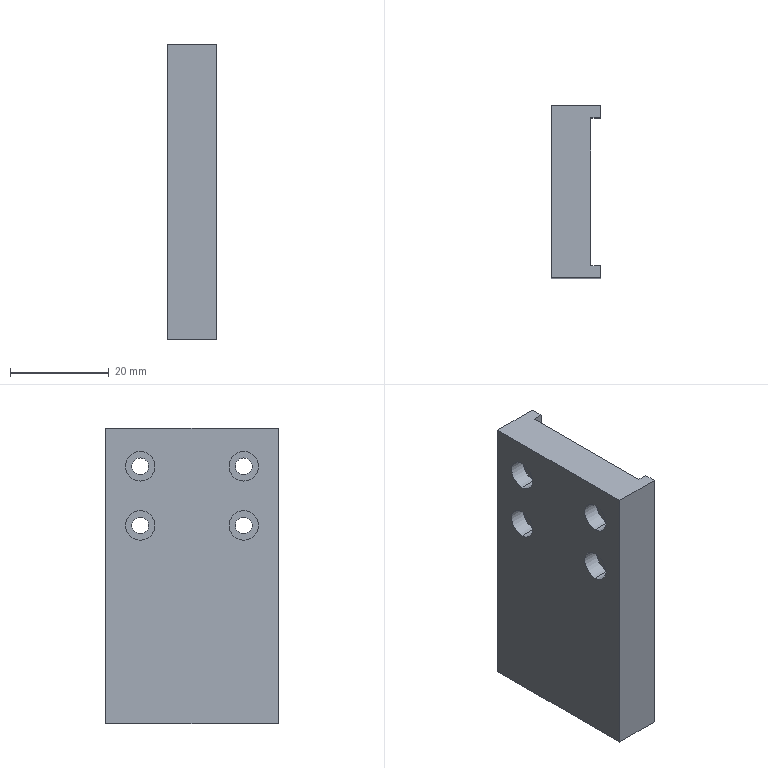Part | SolidWorks | features HoleWzd 2, Cut 1, Extrusion 1 | 1 solid | 38 faces | box 10 x 35 x 60 mm | volume 16670 mm3 | cylinder 20 | plane 14 | cone 4 | commonest cylinder face diameters 3.4 x8 6 x8 3.3 x4
STEP:
#1=CARTESIAN_POINT('',(5.65,10.,-19.9));
#2=VERTEX_POINT('',#1);
#3=CARTESIAN_POINT('',(2.35,10.,-19.9));
#4=VERTEX_POINT('',#3);
#5=CARTESIAN_POINT('',(4.,10.,-19.9));
#6=DIRECTION('',(0.,0.,-1.));
#7=DIRECTION('',(-1.,0.,0.));
#8=AXIS2_PLACEMENT_3D('',#5,#6,#7);
#9=CIRCLE('',#8,1.65);
#10=EDGE_CURVE('',#2,#4,#9,.T.);
#11=ORIENTED_EDGE('',*,*,#10,.F.);
#12=CARTESIAN_POINT('',(5.65,10.,-30.));
#13=VERTEX_POINT('',#12);
#14=CARTESIAN_POINT('',(5.65,10.,-30.));
#15=DIRECTION('',(0.,0.,-1.));
#16=VECTOR('',#15,1000.);
#17=LINE('',#14,#16);
#18=EDGE_CURVE('',#2,#13,#17,.T.);
#19=ORIENTED_EDGE('',*,*,#18,.T.);
#20=CARTESIAN_POINT('',(2.35,10.,-30.));
#21=VERTEX_POINT('',#20);
#22=CARTESIAN_POINT('',(4.,10.,-30.));
#23=DIRECTION('',(0.,0.,-1.));
#24=DIRECTION('',(-1.,0.,0.));
#25=AXIS2_PLACEMENT_3D('',#22,#23,#24);
#26=CIRCLE('',#25,1.65);
#27=EDGE_CURVE('',#13,#21,#26,.T.);
#28=ORIENTED_EDGE('',*,*,#27,.T.);
#29=CARTESIAN_POINT('',(2.35,10.,-30.));
#30=DIRECTION('',(0.,0.,-1.));
#31=VECTOR('',#30,1000.);
#32=LINE('',#29,#31);
#33=EDGE_CURVE('',#4,#21,#32,.T.);
#34=ORIENTED_EDGE('',*,*,#33,.F.);
#35=EDGE_LOOP('',(#11,#19,#28,#34));
#36=FACE_OUTER_BOUND('',#35,.T.);
#37=CARTESIAN_POINT('',(4.,10.,-30.));
#38=DIRECTION('',(0.,0.,-1.));
#39=DIRECTION('',(-1.,0.,0.));
#40=AXIS2_PLACEMENT_3D('',#37,#38,#39);
#41=CYLINDRICAL_SURFACE('',#40,1.65);
#42=ADVANCED_FACE('',(#36),#41,.F.);
#43=CARTESIAN_POINT('',(4.,10.,-18.909));
#44=VERTEX_POINT('',#43);
#45=CARTESIAN_POINT('',(2.35,10.,-19.9));
#46=DIRECTION('',(-0.8572,0.,-0.515));
#47=VECTOR('',#46,1000.);
#48=LINE('',#45,#47);
#49=EDGE_CURVE('',#44,#4,#48,.T.);
#50=ORIENTED_EDGE('',*,*,#49,.F.);
#51=CARTESIAN_POINT('',(5.65,10.,-19.9));
#52=DIRECTION('',(0.8572,0.,-0.515));
#53=VECTOR('',#52,1000.);
#54=LINE('',#51,#53);
#55=EDGE_CURVE('',#44,#2,#54,.T.);
#56=ORIENTED_EDGE('',*,*,#55,.T.);
#57=ORIENTED_EDGE('',*,*,#10,.T.);
#58=EDGE_LOOP('',(#50,#56,#57));
#59=FACE_OUTER_BOUND('',#58,.T.);
#60=CARTESIAN_POINT('',(4.,10.,-19.9));
#61=DIRECTION('',(0.,0.,-1.));
#62=DIRECTION('',(-1.,0.,0.));
#63=AXIS2_PLACEMENT_3D('',#60,#61,#62);
#64=CONICAL_SURFACE('',#63,1.65,1.03);
#65=ADVANCED_FACE('',(#59),#64,.F.);
#66=CARTESIAN_POINT('',(5.65,-10.,-19.9));
#67=VERTEX_POINT('',#66);
#68=CARTESIAN_POINT('',(2.35,-10.,-19.9));
#69=VERTEX_POINT('',#68);
#70=CARTESIAN_POINT('',(4.,-10.,-19.9));
#71=DIRECTION('',(0.,0.,-1.));
#72=DIRECTION('',(-1.,0.,0.));
#73=AXIS2_PLACEMENT_3D('',#70,#71,#72);
#74=CIRCLE('',#73,1.65);
#75=EDGE_CURVE('',#67,#69,#74,.T.);
#76=ORIENTED_EDGE('',*,*,#75,.F.);
#77=CARTESIAN_POINT('',(5.65,-10.,-30.));
#78=VERTEX_POINT('',#77);
#79=CARTESIAN_POINT('',(5.65,-10.,-30.));
#80=DIRECTION('',(0.,0.,-1.));
#81=VECTOR('',#80,1000.);
#82=LINE('',#79,#81);
#83=EDGE_CURVE('',#67,#78,#82,.T.);
#84=ORIENTED_EDGE('',*,*,#83,.T.);
#85=CARTESIAN_POINT('',(2.35,-10.,-30.));
#86=VERTEX_POINT('',#85);
#87=CARTESIAN_POINT('',(4.,-10.,-30.));
#88=DIRECTION('',(0.,0.,-1.));
#89=DIRECTION('',(-1.,0.,0.));
#90=AXIS2_PLACEMENT_3D('',#87,#88,#89);
#91=CIRCLE('',#90,1.65);
#92=EDGE_CURVE('',#78,#86,#91,.T.);
#93=ORIENTED_EDGE('',*,*,#92,.T.);
#94=CARTESIAN_POINT('',(2.35,-10.,-30.));
#95=DIRECTION('',(0.,0.,-1.));
#96=VECTOR('',#95,1000.);
#97=LINE('',#94,#96);
#98=EDGE_CURVE('',#69,#86,#97,.T.);
#99=ORIENTED_EDGE('',*,*,#98,.F.);
#100=EDGE_LOOP('',(#76,#84,#93,#99));
#101=FACE_OUTER_BOUND('',#100,.T.);
#102=CARTESIAN_POINT('',(4.,-10.,-30.));
#103=DIRECTION('',(0.,0.,-1.));
#104=DIRECTION('',(-1.,0.,0.));
#105=AXIS2_PLACEMENT_3D('',#102,#103,#104);
#106=CYLINDRICAL_SURFACE('',#105,1.65);
#107=ADVANCED_FACE('',(#101),#106,.F.);
#108=CARTESIAN_POINT('',(4.,-10.,-18.909));
#109=VERTEX_POINT('',#108);
#110=CARTESIAN_POINT('',(2.35,-10.,-19.9));
#111=DIRECTION('',(-0.8572,0.,-0.515));
#112=VECTOR('',#111,1000.);
#113=LINE('',#110,#112);
#114=EDGE_CURVE('',#109,#69,#113,.T.);
#115=ORIENTED_EDGE('',*,*,#114,.F.);
#116=CARTESIAN_POINT('',(5.65,-10.,-19.9));
#117=DIRECTION('',(0.8572,0.,-0.515));
#118=VECTOR('',#117,1000.);
#119=LINE('',#116,#118);
#120=EDGE_CURVE('',#109,#67,#119,.T.);
#121=ORIENTED_EDGE('',*,*,#120,.T.);
#122=ORIENTED_EDGE('',*,*,#75,.T.);
#123=EDGE_LOOP('',(#115,#121,#122));
#124=FACE_OUTER_BOUND('',#123,.T.);
#125=CARTESIAN_POINT('',(4.,-10.,-19.9));
#126=DIRECTION('',(0.,0.,-1.));
#127=DIRECTION('',(-1.,0.,0.));
#128=AXIS2_PLACEMENT_3D('',#125,#126,#127);
#129=CONICAL_SURFACE('',#128,1.65,1.03);
#130=ADVANCED_FACE('',(#124),#129,.F.);
#131=CARTESIAN_POINT('',(3.4,10.5,19.25));
#132=VERTEX_POINT('',#131);
#133=CARTESIAN_POINT('',(3.4,10.5,25.25));
#134=VERTEX_POINT('',#133);
#135=CARTESIAN_POINT('',(3.4,10.5,22.25));
#136=DIRECTION('',(-1.,0.,0.));
#137=DIRECTION('',(0.,0.,1.));
#138=AXIS2_PLACEMENT_3D('',#135,#136,#137);
#139=CIRCLE('',#138,3.);
#140=EDGE_CURVE('',#132,#134,#139,.T.);
#141=ORIENTED_EDGE('',*,*,#140,.F.);
#142=CARTESIAN_POINT('',(0.,10.5,19.25));
#143=VERTEX_POINT('',#142);
#144=CARTESIAN_POINT('',(0.,10.5,19.25));
#145=DIRECTION('',(-1.,0.,0.));
#146=VECTOR('',#145,1000.);
#147=LINE('',#144,#146);
#148=EDGE_CURVE('',#132,#143,#147,.T.);
#149=ORIENTED_EDGE('',*,*,#148,.T.);
#150=CARTESIAN_POINT('',(0.,10.5,25.25));
#151=VERTEX_POINT('',#150);
#152=CARTESIAN_POINT('',(0.,10.5,22.25));
#153=DIRECTION('',(-1.,0.,0.));
#154=DIRECTION('',(0.,0.,1.));
#155=AXIS2_PLACEMENT_3D('',#152,#153,#154);
#156=CIRCLE('',#155,3.);
#157=EDGE_CURVE('',#143,#151,#156,.T.);
#158=ORIENTED_EDGE('',*,*,#157,.T.);
#159=CARTESIAN_POINT('',(0.,10.5,25.25));
#160=DIRECTION('',(-1.,0.,0.));
#161=VECTOR('',#160,1000.);
#162=LINE('',#159,#161);
#163=EDGE_CURVE('',#134,#151,#162,.T.);
#164=ORIENTED_EDGE('',*,*,#163,.F.);
#165=EDGE_LOOP('',(#141,#149,#158,#164));
#166=FACE_OUTER_BOUND('',#165,.T.);
#167=CARTESIAN_POINT('',(0.,10.5,22.25));
#168=DIRECTION('',(-1.,0.,0.));
#169=DIRECTION('',(0.,0.,1.));
#170=AXIS2_PLACEMENT_3D('',#167,#168,#169);
#171=CYLINDRICAL_SURFACE('',#170,3.);
#172=ADVANCED_FACE('',(#166),#171,.F.);
#173=CARTESIAN_POINT('',(8.,10.5,23.95));
#174=VERTEX_POINT('',#173);
#175=CARTESIAN_POINT('',(8.,10.5,20.55));
#176=VERTEX_POINT('',#175);
#177=CARTESIAN_POINT('',(8.,10.5,22.25));
#178=DIRECTION('',(1.,0.,0.));
#179=DIRECTION('',(0.,0.,-1.));
#180=AXIS2_PLACEMENT_3D('',#177,#178,#179);
#181=CIRCLE('',#180,1.7);
#182=EDGE_CURVE('',#174,#176,#181,.T.);
#183=ORIENTED_EDGE('',*,*,#182,.T.);
#184=CARTESIAN_POINT('',(3.4,10.5,20.55));
#185=VERTEX_POINT('',#184);
#186=CARTESIAN_POINT('',(0.,10.5,20.55));
#187=DIRECTION('',(-1.,0.,0.));
#188=VECTOR('',#187,1000.);
#189=LINE('',#186,#188);
#190=EDGE_CURVE('',#176,#185,#189,.T.);
#191=ORIENTED_EDGE('',*,*,#190,.T.);
#192=CARTESIAN_POINT('',(3.4,10.5,23.95));
#193=VERTEX_POINT('',#192);
#194=CARTESIAN_POINT('',(3.4,10.5,22.25));
#195=DIRECTION('',(-1.,0.,0.));
#196=DIRECTION('',(0.,0.,1.));
#197=AXIS2_PLACEMENT_3D('',#194,#195,#196);
#198=CIRCLE('',#197,1.7);
#199=EDGE_CURVE('',#185,#193,#198,.T.);
#200=ORIENTED_EDGE('',*,*,#199,.T.);
#201=CARTESIAN_POINT('',(0.,10.5,23.95));
#202=DIRECTION('',(-1.,0.,0.));
#203=VECTOR('',#202,1000.);
#204=LINE('',#201,#203);
#205=EDGE_CURVE('',#174,#193,#204,.T.);
#206=ORIENTED_EDGE('',*,*,#205,.F.);
#207=EDGE_LOOP('',(#183,#191,#200,#206));
#208=FACE_OUTER_BOUND('',#207,.T.);
#209=CARTESIAN_POINT('',(0.,10.5,22.25));
#210=DIRECTION('',(-1.,0.,0.));
#211=DIRECTION('',(0.,0.,1.));
#212=AXIS2_PLACEMENT_3D('',#209,#210,#211);
#213=CYLINDRICAL_SURFACE('',#212,1.7);
#214=ADVANCED_FACE('',(#208),#213,.F.);
#215=CARTESIAN_POINT('',(3.4,10.5,7.25));
#216=VERTEX_POINT('',#215);
#217=CARTESIAN_POINT('',(3.4,10.5,13.25));
#218=VERTEX_POINT('',#217);
#219=CARTESIAN_POINT('',(3.4,10.5,10.25));
#220=DIRECTION('',(-1.,0.,0.));
#221=DIRECTION('',(0.,0.,1.));
#222=AXIS2_PLACEMENT_3D('',#219,#220,#221);
#223=CIRCLE('',#222,3.);
#224=EDGE_CURVE('',#216,#218,#223,.T.);
#225=ORIENTED_EDGE('',*,*,#224,.F.);
#226=CARTESIAN_POINT('',(0.,10.5,7.25));
#227=VERTEX_POINT('',#226);
#228=CARTESIAN_POINT('',(0.,10.5,7.25));
#229=DIRECTION('',(-1.,0.,0.));
#230=VECTOR('',#229,1000.);
#231=LINE('',#228,#230);
#232=EDGE_CURVE('',#216,#227,#231,.T.);
#233=ORIENTED_EDGE('',*,*,#232,.T.);
#234=CARTESIAN_POINT('',(0.,10.5,13.25));
#235=VERTEX_POINT('',#234);
#236=CARTESIAN_POINT('',(0.,10.5,10.25));
#237=DIRECTION('',(-1.,0.,0.));
#238=DIRECTION('',(0.,0.,1.));
#239=AXIS2_PLACEMENT_3D('',#236,#237,#238);
#240=CIRCLE('',#239,3.);
#241=EDGE_CURVE('',#227,#235,#240,.T.);
#242=ORIENTED_EDGE('',*,*,#241,.T.);
#243=CARTESIAN_POINT('',(0.,10.5,13.25));
#244=DIRECTION('',(-1.,0.,0.));
#245=VECTOR('',#244,1000.);
#246=LINE('',#243,#245);
#247=EDGE_CURVE('',#218,#235,#246,.T.);
#248=ORIENTED_EDGE('',*,*,#247,.F.);
#249=EDGE_LOOP('',(#225,#233,#242,#248));
#250=FACE_OUTER_BOUND('',#249,.T.);
#251=CARTESIAN_POINT('',(0.,10.5,10.25));
#252=DIRECTION('',(-1.,0.,0.));
#253=DIRECTION('',(0.,0.,1.));
#254=AXIS2_PLACEMENT_3D('',#251,#252,#253);
#255=CYLINDRICAL_SURFACE('',#254,3.);
#256=ADVANCED_FACE('',(#250),#255,.F.);
#257=CARTESIAN_POINT('',(8.,10.5,11.95));
#258=VERTEX_POINT('',#257);
#259=CARTESIAN_POINT('',(8.,10.5,8.55));
#260=VERTEX_POINT('',#259);
#261=CARTESIAN_POINT('',(8.,10.5,10.25));
#262=DIRECTION('',(1.,0.,0.));
#263=DIRECTION('',(0.,0.,-1.));
#264=AXIS2_PLACEMENT_3D('',#261,#262,#263);
#265=CIRCLE('',#264,1.7);
#266=EDGE_CURVE('',#258,#260,#265,.T.);
#267=ORIENTED_EDGE('',*,*,#266,.T.);
#268=CARTESIAN_POINT('',(3.4,10.5,8.55));
#269=VERTEX_POINT('',#268);
#270=CARTESIAN_POINT('',(0.,10.5,8.55));
#271=DIRECTION('',(-1.,0.,0.));
#272=VECTOR('',#271,1000.);
#273=LINE('',#270,#272);
#274=EDGE_CURVE('',#260,#269,#273,.T.);
#275=ORIENTED_EDGE('',*,*,#274,.T.);
#276=CARTESIAN_POINT('',(3.4,10.5,11.95));
#277=VERTEX_POINT('',#276);
#278=CARTESIAN_POINT('',(3.4,10.5,10.25));
#279=DIRECTION('',(-1.,0.,0.));
#280=DIRECTION('',(0.,0.,1.));
#281=AXIS2_PLACEMENT_3D('',#278,#279,#280);
#282=CIRCLE('',#281,1.7);
#283=EDGE_CURVE('',#269,#277,#282,.T.);
#284=ORIENTED_EDGE('',*,*,#283,.T.);
#285=CARTESIAN_POINT('',(0.,10.5,11.95));
#286=DIRECTION('',(-1.,0.,0.));
#287=VECTOR('',#286,1000.);
#288=LINE('',#285,#287);
#289=EDGE_CURVE('',#258,#277,#288,.T.);
#290=ORIENTED_EDGE('',*,*,#289,.F.);
#291=EDGE_LOOP('',(#267,#275,#284,#290));
#292=FACE_OUTER_BOUND('',#291,.T.);
#293=CARTESIAN_POINT('',(0.,10.5,10.25));
#294=DIRECTION('',(-1.,0.,0.));
#295=DIRECTION('',(0.,0.,1.));
#296=AXIS2_PLACEMENT_3D('',#293,#294,#295);
#297=CYLINDRICAL_SURFACE('',#296,1.7);
#298=ADVANCED_FACE('',(#292),#297,.F.);
#299=CARTESIAN_POINT('',(3.4,-10.5,7.25));
#300=VERTEX_POINT('',#299);
#301=CARTESIAN_POINT('',(3.4,-10.5,13.25));
#302=VERTEX_POINT('',#301);
#303=CARTESIAN_POINT('',(3.4,-10.5,10.25));
#304=DIRECTION('',(-1.,0.,0.));
#305=DIRECTION('',(0.,0.,1.));
#306=AXIS2_PLACEMENT_3D('',#303,#304,#305);
#307=CIRCLE('',#306,3.);
#308=EDGE_CURVE('',#300,#302,#307,.T.);
#309=ORIENTED_EDGE('',*,*,#308,.F.);
#310=CARTESIAN_POINT('',(0.,-10.5,7.25));
#311=VERTEX_POINT('',#310);
#312=CARTESIAN_POINT('',(0.,-10.5,7.25));
#313=DIRECTION('',(-1.,0.,0.));
#314=VECTOR('',#313,1000.);
#315=LINE('',#312,#314);
#316=EDGE_CURVE('',#300,#311,#315,.T.);
#317=ORIENTED_EDGE('',*,*,#316,.T.);
#318=CARTESIAN_POINT('',(0.,-10.5,13.25));
#319=VERTEX_POINT('',#318);
#320=CARTESIAN_POINT('',(0.,-10.5,10.25));
#321=DIRECTION('',(-1.,0.,0.));
#322=DIRECTION('',(0.,0.,1.));
#323=AXIS2_PLACEMENT_3D('',#320,#321,#322);
#324=CIRCLE('',#323,3.);
#325=EDGE_CURVE('',#311,#319,#324,.T.);
#326=ORIENTED_EDGE('',*,*,#325,.T.);
#327=CARTESIAN_POINT('',(0.,-10.5,13.25));
#328=DIRECTION('',(-1.,0.,0.));
#329=VECTOR('',#328,1000.);
#330=LINE('',#327,#329);
#331=EDGE_CURVE('',#302,#319,#330,.T.);
#332=ORIENTED_EDGE('',*,*,#331,.F.);
#333=EDGE_LOOP('',(#309,#317,#326,#332));
#334=FACE_OUTER_BOUND('',#333,.T.);
#335=CARTESIAN_POINT('',(0.,-10.5,10.25));
#336=DIRECTION('',(-1.,0.,0.));
#337=DIRECTION('',(0.,0.,1.));
#338=AXIS2_PLACEMENT_3D('',#335,#336,#337);
#339=CYLINDRICAL_SURFACE('',#338,3.);
#340=ADVANCED_FACE('',(#334),#339,.F.);
#341=CARTESIAN_POINT('',(8.,-10.5,11.95));
#342=VERTEX_POINT('',#341);
#343=CARTESIAN_POINT('',(8.,-10.5,8.55));
#344=VERTEX_POINT('',#343);
#345=CARTESIAN_POINT('',(8.,-10.5,10.25));
#346=DIRECTION('',(1.,0.,0.));
#347=DIRECTION('',(0.,0.,-1.));
#348=AXIS2_PLACEMENT_3D('',#345,#346,#347);
#349=CIRCLE('',#348,1.7);
#350=EDGE_CURVE('',#342,#344,#349,.T.);
#351=ORIENTED_EDGE('',*,*,#350,.T.);
#352=CARTESIAN_POINT('',(3.4,-10.5,8.55));
#353=VERTEX_POINT('',#352);
#354=CARTESIAN_POINT('',(0.,-10.5,8.55));
#355=DIRECTION('',(-1.,0.,0.));
#356=VECTOR('',#355,1000.);
#357=LINE('',#354,#356);
#358=EDGE_CURVE('',#344,#353,#357,.T.);
#359=ORIENTED_EDGE('',*,*,#358,.T.);
#360=CARTESIAN_POINT('',(3.4,-10.5,11.95));
#361=VERTEX_POINT('',#360);
#362=CARTESIAN_POINT('',(3.4,-10.5,10.25));
#363=DIRECTION('',(-1.,0.,0.));
#364=DIRECTION('',(0.,0.,1.));
#365=AXIS2_PLACEMENT_3D('',#362,#363,#364);
#366=CIRCLE('',#365,1.7);
#367=EDGE_CURVE('',#353,#361,#366,.T.);
#368=ORIENTED_EDGE('',*,*,#367,.T.);
#369=CARTESIAN_POINT('',(0.,-10.5,11.95));
#370=DIRECTION('',(-1.,0.,0.));
#371=VECTOR('',#370,1000.);
#372=LINE('',#369,#371);
#373=EDGE_CURVE('',#342,#361,#372,.T.);
#374=ORIENTED_EDGE('',*,*,#373,.F.);
#375=EDGE_LOOP('',(#351,#359,#368,#374));
#376=FACE_OUTER_BOUND('',#375,.T.);
#377=CARTESIAN_POINT('',(0.,-10.5,10.25));
#378=DIRECTION('',(-1.,0.,0.));
#379=DIRECTION('',(0.,0.,1.));
#380=AXIS2_PLACEMENT_3D('',#377,#378,#379);
#381=CYLINDRICAL_SURFACE('',#380,1.7);
#382=ADVANCED_FACE('',(#376),#381,.F.);
#383=CARTESIAN_POINT('',(3.4,-10.5,19.25));
#384=VERTEX_POINT('',#383);
#385=CARTESIAN_POINT('',(3.4,-10.5,25.25));
#386=VERTEX_POINT('',#385);
#387=CARTESIAN_POINT('',(3.4,-10.5,22.25));
#388=DIRECTION('',(-1.,0.,0.));
#389=DIRECTION('',(0.,0.,1.));
#390=AXIS2_PLACEMENT_3D('',#387,#388,#389);
#391=CIRCLE('',#390,3.);
#392=EDGE_CURVE('',#384,#386,#391,.T.);
#393=ORIENTED_EDGE('',*,*,#392,.F.);
#394=CARTESIAN_POINT('',(0.,-10.5,19.25));
#395=VERTEX_POINT('',#394);
#396=CARTESIAN_POINT('',(0.,-10.5,19.25));
#397=DIRECTION('',(-1.,0.,0.));
#398=VECTOR('',#397,1000.);
#399=LINE('',#396,#398);
#400=EDGE_CURVE('',#384,#395,#399,.T.);
#401=ORIENTED_EDGE('',*,*,#400,.T.);
#402=CARTESIAN_POINT('',(0.,-10.5,25.25));
#403=VERTEX_POINT('',#402);
#404=CARTESIAN_POINT('',(0.,-10.5,22.25));
#405=DIRECTION('',(-1.,0.,0.));
#406=DIRECTION('',(0.,0.,1.));
#407=AXIS2_PLACEMENT_3D('',#404,#405,#406);
#408=CIRCLE('',#407,3.);
#409=EDGE_CURVE('',#395,#403,#408,.T.);
#410=ORIENTED_EDGE('',*,*,#409,.T.);
#411=CARTESIAN_POINT('',(0.,-10.5,25.25));
#412=DIRECTION('',(-1.,0.,0.));
#413=VECTOR('',#412,1000.);
#414=LINE('',#411,#413);
#415=EDGE_CURVE('',#386,#403,#414,.T.);
#416=ORIENTED_EDGE('',*,*,#415,.F.);
#417=EDGE_LOOP('',(#393,#401,#410,#416));
#418=FACE_OUTER_BOUND('',#417,.T.);
#419=CARTESIAN_POINT('',(0.,-10.5,22.25));
#420=DIRECTION('',(-1.,0.,0.));
#421=DIRECTION('',(0.,0.,1.));
#422=AXIS2_PLACEMENT_3D('',#419,#420,#421);
#423=CYLINDRICAL_SURFACE('',#422,3.);
#424=ADVANCED_FACE('',(#418),#423,.F.);
#425=CARTESIAN_POINT('',(8.,-10.5,23.95));
#426=VERTEX_POINT('',#425);
#427=CARTESIAN_POINT('',(8.,-10.5,20.55));
#428=VERTEX_POINT('',#427);
#429=CARTESIAN_POINT('',(8.,-10.5,22.25));
#430=DIRECTION('',(1.,0.,0.));
#431=DIRECTION('',(0.,0.,-1.));
#432=AXIS2_PLACEMENT_3D('',#429,#430,#431);
#433=CIRCLE('',#432,1.7);
#434=EDGE_CURVE('',#426,#428,#433,.T.);
#435=ORIENTED_EDGE('',*,*,#434,.T.);
#436=CARTESIAN_POINT('',(3.4,-10.5,20.55));
#437=VERTEX_POINT('',#436);
#438=CARTESIAN_POINT('',(0.,-10.5,20.55));
#439=DIRECTION('',(-1.,0.,0.));
#440=VECTOR('',#439,1000.);
#441=LINE('',#438,#440);
#442=EDGE_CURVE('',#428,#437,#441,.T.);
#443=ORIENTED_EDGE('',*,*,#442,.T.);
#444=CARTESIAN_POINT('',(3.4,-10.5,23.95));
#445=VERTEX_POINT('',#444);
#446=CARTESIAN_POINT('',(3.4,-10.5,22.25));
#447=DIRECTION('',(-1.,0.,0.));
#448=DIRECTION('',(0.,0.,1.));
#449=AXIS2_PLACEMENT_3D('',#446,#447,#448);
#450=CIRCLE('',#449,1.7);
#451=EDGE_CURVE('',#437,#445,#450,.T.);
#452=ORIENTED_EDGE('',*,*,#451,.T.);
#453=CARTESIAN_POINT('',(0.,-10.5,23.95));
#454=DIRECTION('',(-1.,0.,0.));
#455=VECTOR('',#454,1000.);
#456=LINE('',#453,#455);
#457=EDGE_CURVE('',#426,#445,#456,.T.);
#458=ORIENTED_EDGE('',*,*,#457,.F.);
#459=EDGE_LOOP('',(#435,#443,#452,#458));
#460=FACE_OUTER_BOUND('',#459,.T.);
#461=CARTESIAN_POINT('',(0.,-10.5,22.25));
#462=DIRECTION('',(-1.,0.,0.));
#463=DIRECTION('',(0.,0.,1.));
#464=AXIS2_PLACEMENT_3D('',#461,#462,#463);
#465=CYLINDRICAL_SURFACE('',#464,1.7);
#466=ADVANCED_FACE('',(#460),#465,.F.);
#467=CARTESIAN_POINT('',(10.,-17.5,-30.));
#468=VERTEX_POINT('',#467);
#469=CARTESIAN_POINT('',(10.,-15.,-30.));
#470=VERTEX_POINT('',#469);
#471=CARTESIAN_POINT('',(10.,-17.5,-30.));
#472=DIRECTION('',(0.,1.,0.));
#473=VECTOR('',#472,1000.);
#474=LINE('',#471,#473);
#475=EDGE_CURVE('',#468,#470,#474,.T.);
#476=ORIENTED_EDGE('',*,*,#475,.T.);
#477=CARTESIAN_POINT('',(10.,-15.,30.));
#478=VERTEX_POINT('',#477);
#479=CARTESIAN_POINT('',(10.,-15.,30.));
#480=DIRECTION('',(0.,0.,-1.));
#481=VECTOR('',#480,1000.);
#482=LINE('',#479,#481);
#483=EDGE_CURVE('',#478,#470,#482,.T.);
#484=ORIENTED_EDGE('',*,*,#483,.F.);
#485=CARTESIAN_POINT('',(10.,-17.5,30.));
#486=VERTEX_POINT('',#485);
#487=CARTESIAN_POINT('',(10.,-17.5,30.));
#488=DIRECTION('',(0.,-1.,0.));
#489=VECTOR('',#488,1000.);
#490=LINE('',#487,#489);
#491=EDGE_CURVE('',#478,#486,#490,.T.);
#492=ORIENTED_EDGE('',*,*,#491,.T.);
#493=CARTESIAN_POINT('',(10.,-17.5,30.));
#494=DIRECTION('',(0.,0.,-1.));
#495=VECTOR('',#494,1000.);
#496=LINE('',#493,#495);
#497=EDGE_CURVE('',#486,#468,#496,.T.);
#498=ORIENTED_EDGE('',*,*,#497,.T.);
#499=EDGE_LOOP('',(#476,#484,#492,#498));
#500=FACE_OUTER_BOUND('',#499,.T.);
#501=CARTESIAN_POINT('',(10.,0.,0.));
#502=DIRECTION('',(-1.,0.,0.));
#503=DIRECTION('',(0.,0.,1.));
#504=AXIS2_PLACEMENT_3D('',#501,#502,#503);
#505=PLANE('',#504);
#506=ADVANCED_FACE('',(#500),#505,.F.);
#507=CARTESIAN_POINT('',(4.,10.,-30.));
#508=DIRECTION('',(0.,0.,-1.));
#509=DIRECTION('',(-1.,0.,0.));
#510=AXIS2_PLACEMENT_3D('',#507,#508,#509);
#511=CIRCLE('',#510,1.65);
#512=EDGE_CURVE('',#21,#13,#511,.T.);
#513=ORIENTED_EDGE('',*,*,#512,.F.);
#514=ORIENTED_EDGE('',*,*,#27,.F.);
#515=EDGE_LOOP('',(#513,#514));
#516=FACE_BOUND('',#515,.T.);
#517=CARTESIAN_POINT('',(4.,-10.,-30.));
#518=DIRECTION('',(0.,0.,-1.));
#519=DIRECTION('',(-1.,0.,0.));
#520=AXIS2_PLACEMENT_3D('',#517,#518,#519);
#521=CIRCLE('',#520,1.65);
#522=EDGE_CURVE('',#86,#78,#521,.T.);
#523=ORIENTED_EDGE('',*,*,#522,.F.);
#524=ORIENTED_EDGE('',*,*,#92,.F.);
#525=EDGE_LOOP('',(#523,#524));
#526=FACE_BOUND('',#525,.T.);
#527=CARTESIAN_POINT('',(8.,-15.,-30.));
#528=VERTEX_POINT('',#527);
#529=CARTESIAN_POINT('',(8.,15.,-30.));
#530=VERTEX_POINT('',#529);
#531=CARTESIAN_POINT('',(8.,15.,-30.));
#532=DIRECTION('',(0.,1.,0.));
#533=VECTOR('',#532,1000.);
#534=LINE('',#531,#533);
#535=EDGE_CURVE('',#528,#530,#534,.T.);
#536=ORIENTED_EDGE('',*,*,#535,.F.);
#537=CARTESIAN_POINT('',(8.,-15.,-30.));
#538=DIRECTION('',(1.,0.,0.));
#539=VECTOR('',#538,1000.);
#540=LINE('',#537,#539);
#541=EDGE_CURVE('',#528,#470,#540,.T.);
#542=ORIENTED_EDGE('',*,*,#541,.T.);
#543=ORIENTED_EDGE('',*,*,#475,.F.);
#544=CARTESIAN_POINT('',(0.,-17.5,-30.));
#545=VERTEX_POINT('',#544);
#546=CARTESIAN_POINT('',(10.,-17.5,-30.));
#547=DIRECTION('',(-1.,0.,0.));
#548=VECTOR('',#547,1000.);
#549=LINE('',#546,#548);
#550=EDGE_CURVE('',#468,#545,#549,.T.);
#551=ORIENTED_EDGE('',*,*,#550,.T.);
#552=CARTESIAN_POINT('',(0.,17.5,-30.));
#553=VERTEX_POINT('',#552);
#554=CARTESIAN_POINT('',(0.,-17.5,-30.));
#555=DIRECTION('',(0.,1.,0.));
#556=VECTOR('',#555,1000.);
#557=LINE('',#554,#556);
#558=EDGE_CURVE('',#545,#553,#557,.T.);
#559=ORIENTED_EDGE('',*,*,#558,.T.);
#560=CARTESIAN_POINT('',(10.,17.5,-30.));
#561=VERTEX_POINT('',#560);
#562=CARTESIAN_POINT('',(10.,17.5,-30.));
#563=DIRECTION('',(-1.,0.,0.));
#564=VECTOR('',#563,1000.);
#565=LINE('',#562,#564);
#566=EDGE_CURVE('',#561,#553,#565,.T.);
#567=ORIENTED_EDGE('',*,*,#566,.F.);
#568=CARTESIAN_POINT('',(10.,15.,-30.));
#569=VERTEX_POINT('',#568);
#570=CARTESIAN_POINT('',(10.,-17.5,-30.));
#571=DIRECTION('',(0.,1.,0.));
#572=VECTOR('',#571,1000.);
#573=LINE('',#570,#572);
#574=EDGE_CURVE('',#569,#561,#573,.T.);
#575=ORIENTED_EDGE('',*,*,#574,.F.);
#576=CARTESIAN_POINT('',(8.,15.,-30.));
#577=DIRECTION('',(1.,0.,0.));
#578=VECTOR('',#577,1000.);
#579=LINE('',#576,#578);
#580=EDGE_CURVE('',#530,#569,#579,.T.);
#581=ORIENTED_EDGE('',*,*,#580,.F.);
#582=EDGE_LOOP('',(#536,#542,#543,#551,#559,#567,#575,#581));
#583=FACE_OUTER_BOUND('',#582,.T.);
#584=CARTESIAN_POINT('',(10.,-17.5,-30.));
#585=DIRECTION('',(0.,0.,1.));
#586=DIRECTION('',(1.,0.,0.));
#587=AXIS2_PLACEMENT_3D('',#584,#585,#586);
#588=PLANE('',#587);
#589=ADVANCED_FACE('',(#516,#526,#583),#588,.F.);
#590=CARTESIAN_POINT('',(0.,17.5,30.));
#591=VERTEX_POINT('',#590);
#592=CARTESIAN_POINT('',(0.,17.5,30.));
#593=DIRECTION('',(0.,0.,1.));
#594=VECTOR('',#593,1000.);
#595=LINE('',#592,#594);
#596=EDGE_CURVE('',#553,#591,#595,.T.);
#597=ORIENTED_EDGE('',*,*,#596,.T.);
#598=CARTESIAN_POINT('',(10.,17.5,30.));
#599=VERTEX_POINT('',#598);
#600=CARTESIAN_POINT('',(10.,17.5,30.));
#601=DIRECTION('',(-1.,0.,0.));
#602=VECTOR('',#601,1000.);
#603=LINE('',#600,#602);
#604=EDGE_CURVE('',#599,#591,#603,.T.);
#605=ORIENTED_EDGE('',*,*,#604,.F.);
#606=CARTESIAN_POINT('',(10.,17.5,30.));
#607=DIRECTION('',(0.,0.,1.));
#608=VECTOR('',#607,1000.);
#609=LINE('',#606,#608);
#610=EDGE_CURVE('',#561,#599,#609,.T.);
#611=ORIENTED_EDGE('',*,*,#610,.F.);
#612=ORIENTED_EDGE('',*,*,#566,.T.);
#613=EDGE_LOOP('',(#597,#605,#611,#612));
#614=FACE_OUTER_BOUND('',#613,.T.);
#615=CARTESIAN_POINT('',(10.,17.5,30.));
#616=DIRECTION('',(0.,-1.,0.));
#617=DIRECTION('',(0.,0.,-1.));
#618=AXIS2_PLACEMENT_3D('',#615,#616,#617);
#619=PLANE('',#618);
#620=ADVANCED_FACE('',(#614),#619,.F.);
#621=ORIENTED_EDGE('',*,*,#491,.F.);
#622=CARTESIAN_POINT('',(8.,-15.,30.));
#623=VERTEX_POINT('',#622);
#624=CARTESIAN_POINT('',(8.,-15.,30.));
#625=DIRECTION('',(1.,0.,0.));
#626=VECTOR('',#625,1000.);
#627=LINE('',#624,#626);
#628=EDGE_CURVE('',#623,#478,#627,.T.);
#629=ORIENTED_EDGE('',*,*,#628,.F.);
#630=CARTESIAN_POINT('',(8.,15.,30.));
#631=VERTEX_POINT('',#630);
#632=CARTESIAN_POINT('',(8.,15.,30.));
#633=DIRECTION('',(0.,-1.,0.));
#634=VECTOR('',#633,1000.);
#635=LINE('',#632,#634);
#636=EDGE_CURVE('',#631,#623,#635,.T.);
#637=ORIENTED_EDGE('',*,*,#636,.F.);
#638=CARTESIAN_POINT('',(10.,15.,30.));
#639=VERTEX_POINT('',#638);
#640=CARTESIAN_POINT('',(8.,15.,30.));
#641=DIRECTION('',(1.,0.,0.));
#642=VECTOR('',#641,1000.);
#643=LINE('',#640,#642);
#644=EDGE_CURVE('',#631,#639,#643,.T.);
#645=ORIENTED_EDGE('',*,*,#644,.T.);
#646=CARTESIAN_POINT('',(10.,-17.5,30.));
#647=DIRECTION('',(0.,-1.,0.));
#648=VECTOR('',#647,1000.);
#649=LINE('',#646,#648);
#650=EDGE_CURVE('',#599,#639,#649,.T.);
#651=ORIENTED_EDGE('',*,*,#650,.F.);
#652=ORIENTED_EDGE('',*,*,#604,.T.);
#653=CARTESIAN_POINT('',(0.,-17.5,30.));
#654=VERTEX_POINT('',#653);
#655=CARTESIAN_POINT('',(0.,-17.5,30.));
#656=DIRECTION('',(0.,-1.,0.));
#657=VECTOR('',#656,1000.);
#658=LINE('',#655,#657);
#659=EDGE_CURVE('',#591,#654,#658,.T.);
#660=ORIENTED_EDGE('',*,*,#659,.T.);
#661=CARTESIAN_POINT('',(10.,-17.5,30.));
#662=DIRECTION('',(-1.,0.,0.));
#663=VECTOR('',#662,1000.);
#664=LINE('',#661,#663);
#665=EDGE_CURVE('',#486,#654,#664,.T.);
#666=ORIENTED_EDGE('',*,*,#665,.F.);
#667=EDGE_LOOP('',(#621,#629,#637,#645,#651,#652,#660,#666));
#668=FACE_OUTER_BOUND('',#667,.T.);
#669=CARTESIAN_POINT('',(10.,-17.5,30.));
#670=DIRECTION('',(0.,0.,-1.));
#671=DIRECTION('',(-1.,0.,0.));
#672=AXIS2_PLACEMENT_3D('',#669,#670,#671);
#673=PLANE('',#672);
#674=ADVANCED_FACE('',(#668),#673,.F.);
#675=CARTESIAN_POINT('',(0.,-17.5,30.));
#676=DIRECTION('',(0.,0.,-1.));
#677=VECTOR('',#676,1000.);
#678=LINE('',#675,#677);
#679=EDGE_CURVE('',#654,#545,#678,.T.);
#680=ORIENTED_EDGE('',*,*,#679,.T.);
#681=ORIENTED_EDGE('',*,*,#550,.F.);
#682=ORIENTED_EDGE('',*,*,#497,.F.);
#683=ORIENTED_EDGE('',*,*,#665,.T.);
#684=EDGE_LOOP('',(#680,#681,#682,#683));
#685=FACE_OUTER_BOUND('',#684,.T.);
#686=CARTESIAN_POINT('',(10.,-17.5,30.));
#687=DIRECTION('',(0.,1.,0.));
#688=DIRECTION('',(0.,0.,1.));
#689=AXIS2_PLACEMENT_3D('',#686,#687,#688);
#690=PLANE('',#689);
#691=ADVANCED_FACE('',(#685),#690,.F.);
#692=ORIENTED_EDGE('',*,*,#650,.T.);
#693=CARTESIAN_POINT('',(10.,15.,30.));
#694=DIRECTION('',(0.,0.,1.));
#695=VECTOR('',#694,1000.);
#696=LINE('',#693,#695);
#697=EDGE_CURVE('',#569,#639,#696,.T.);
#698=ORIENTED_EDGE('',*,*,#697,.F.);
#699=ORIENTED_EDGE('',*,*,#574,.T.);
#700=ORIENTED_EDGE('',*,*,#610,.T.);
#701=EDGE_LOOP('',(#692,#698,#699,#700));
#702=FACE_OUTER_BOUND('',#701,.T.);
#703=CARTESIAN_POINT('',(10.,0.,0.));
#704=DIRECTION('',(-1.,0.,0.));
#705=DIRECTION('',(0.,0.,1.));
#706=AXIS2_PLACEMENT_3D('',#703,#704,#705);
#707=PLANE('',#706);
#708=ADVANCED_FACE('',(#702),#707,.F.);
#709=CARTESIAN_POINT('',(0.,10.5,22.25));
#710=DIRECTION('',(-1.,0.,0.));
#711=DIRECTION('',(0.,0.,1.));
#712=AXIS2_PLACEMENT_3D('',#709,#710,#711);
#713=CIRCLE('',#712,3.);
#714=EDGE_CURVE('',#151,#143,#713,.T.);
#715=ORIENTED_EDGE('',*,*,#714,.F.);
#716=ORIENTED_EDGE('',*,*,#157,.F.);
#717=EDGE_LOOP('',(#715,#716));
#718=FACE_BOUND('',#717,.T.);
#719=CARTESIAN_POINT('',(0.,10.5,10.25));
#720=DIRECTION('',(-1.,0.,0.));
#721=DIRECTION('',(0.,0.,1.));
#722=AXIS2_PLACEMENT_3D('',#719,#720,#721);
#723=CIRCLE('',#722,3.);
#724=EDGE_CURVE('',#235,#227,#723,.T.);
#725=ORIENTED_EDGE('',*,*,#724,.F.);
#726=ORIENTED_EDGE('',*,*,#241,.F.);
#727=EDGE_LOOP('',(#725,#726));
#728=FACE_BOUND('',#727,.T.);
#729=CARTESIAN_POINT('',(0.,-10.5,10.25));
#730=DIRECTION('',(-1.,0.,0.));
#731=DIRECTION('',(0.,0.,1.));
#732=AXIS2_PLACEMENT_3D('',#729,#730,#731);
#733=CIRCLE('',#732,3.);
#734=EDGE_CURVE('',#319,#311,#733,.T.);
#735=ORIENTED_EDGE('',*,*,#734,.F.);
#736=ORIENTED_EDGE('',*,*,#325,.F.);
#737=EDGE_LOOP('',(#735,#736));
#738=FACE_BOUND('',#737,.T.);
#739=CARTESIAN_POINT('',(0.,-10.5,22.25));
#740=DIRECTION('',(-1.,0.,0.));
#741=DIRECTION('',(0.,0.,1.));
#742=AXIS2_PLACEMENT_3D('',#739,#740,#741);
#743=CIRCLE('',#742,3.);
#744=EDGE_CURVE('',#403,#395,#743,.T.);
#745=ORIENTED_EDGE('',*,*,#744,.F.);
#746=ORIENTED_EDGE('',*,*,#409,.F.);
#747=EDGE_LOOP('',(#745,#746));
#748=FACE_BOUND('',#747,.T.);
#749=ORIENTED_EDGE('',*,*,#558,.F.);
#750=ORIENTED_EDGE('',*,*,#679,.F.);
#751=ORIENTED_EDGE('',*,*,#659,.F.);
#752=ORIENTED_EDGE('',*,*,#596,.F.);
#753=EDGE_LOOP('',(#749,#750,#751,#752));
#754=FACE_OUTER_BOUND('',#753,.T.);
#755=CARTESIAN_POINT('',(0.,0.,0.));
#756=DIRECTION('',(-1.,0.,0.));
#757=DIRECTION('',(0.,0.,1.));
#758=AXIS2_PLACEMENT_3D('',#755,#756,#757);
#759=PLANE('',#758);
#760=ADVANCED_FACE('',(#718,#728,#738,#748,#754),#759,.T.);
#761=ORIENTED_EDGE('',*,*,#483,.T.);
#762=ORIENTED_EDGE('',*,*,#541,.F.);
#763=CARTESIAN_POINT('',(8.,-15.,30.));
#764=DIRECTION('',(0.,0.,-1.));
#765=VECTOR('',#764,1000.);
#766=LINE('',#763,#765);
#767=EDGE_CURVE('',#623,#528,#766,.T.);
#768=ORIENTED_EDGE('',*,*,#767,.F.);
#769=ORIENTED_EDGE('',*,*,#628,.T.);
#770=EDGE_LOOP('',(#761,#762,#768,#769));
#771=FACE_OUTER_BOUND('',#770,.T.);
#772=CARTESIAN_POINT('',(8.,-15.,30.));
#773=DIRECTION('',(0.,-1.,0.));
#774=DIRECTION('',(0.,0.,-1.));
#775=AXIS2_PLACEMENT_3D('',#772,#773,#774);
#776=PLANE('',#775);
#777=ADVANCED_FACE('',(#771),#776,.F.);
#778=ORIENTED_EDGE('',*,*,#697,.T.);
#779=ORIENTED_EDGE('',*,*,#644,.F.);
#780=CARTESIAN_POINT('',(8.,15.,30.));
#781=DIRECTION('',(0.,0.,1.));
#782=VECTOR('',#781,1000.);
#783=LINE('',#780,#782);
#784=EDGE_CURVE('',#530,#631,#783,.T.);
#785=ORIENTED_EDGE('',*,*,#784,.F.);
#786=ORIENTED_EDGE('',*,*,#580,.T.);
#787=EDGE_LOOP('',(#778,#779,#785,#786));
#788=FACE_OUTER_BOUND('',#787,.T.);
#789=CARTESIAN_POINT('',(8.,15.,30.));
#790=DIRECTION('',(0.,1.,0.));
#791=DIRECTION('',(0.,0.,1.));
#792=AXIS2_PLACEMENT_3D('',#789,#790,#791);
#793=PLANE('',#792);
#794=ADVANCED_FACE('',(#788),#793,.F.);
#795=ORIENTED_EDGE('',*,*,#182,.F.);
#796=CARTESIAN_POINT('',(8.,10.5,22.25));
#797=DIRECTION('',(1.,0.,0.));
#798=DIRECTION('',(0.,0.,-1.));
#799=AXIS2_PLACEMENT_3D('',#796,#797,#798);
#800=CIRCLE('',#799,1.7);
#801=EDGE_CURVE('',#176,#174,#800,.T.);
#802=ORIENTED_EDGE('',*,*,#801,.F.);
#803=EDGE_LOOP('',(#795,#802));
#804=FACE_BOUND('',#803,.T.);
#805=ORIENTED_EDGE('',*,*,#266,.F.);
#806=CARTESIAN_POINT('',(8.,10.5,10.25));
#807=DIRECTION('',(1.,0.,0.));
#808=DIRECTION('',(0.,0.,-1.));
#809=AXIS2_PLACEMENT_3D('',#806,#807,#808);
#810=CIRCLE('',#809,1.7);
#811=EDGE_CURVE('',#260,#258,#810,.T.);
#812=ORIENTED_EDGE('',*,*,#811,.F.);
#813=EDGE_LOOP('',(#805,#812));
#814=FACE_BOUND('',#813,.T.);
#815=ORIENTED_EDGE('',*,*,#350,.F.);
#816=CARTESIAN_POINT('',(8.,-10.5,10.25));
#817=DIRECTION('',(1.,0.,0.));
#818=DIRECTION('',(0.,0.,-1.));
#819=AXIS2_PLACEMENT_3D('',#816,#817,#818);
#820=CIRCLE('',#819,1.7);
#821=EDGE_CURVE('',#344,#342,#820,.T.);
#822=ORIENTED_EDGE('',*,*,#821,.F.);
#823=EDGE_LOOP('',(#815,#822));
#824=FACE_BOUND('',#823,.T.);
#825=ORIENTED_EDGE('',*,*,#434,.F.);
#826=CARTESIAN_POINT('',(8.,-10.5,22.25));
#827=DIRECTION('',(1.,0.,0.));
#828=DIRECTION('',(0.,0.,-1.));
#829=AXIS2_PLACEMENT_3D('',#826,#827,#828);
#830=CIRCLE('',#829,1.7);
#831=EDGE_CURVE('',#428,#426,#830,.T.);
#832=ORIENTED_EDGE('',*,*,#831,.F.);
#833=EDGE_LOOP('',(#825,#832));
#834=FACE_BOUND('',#833,.T.);
#835=ORIENTED_EDGE('',*,*,#535,.T.);
#836=ORIENTED_EDGE('',*,*,#784,.T.);
#837=ORIENTED_EDGE('',*,*,#636,.T.);
#838=ORIENTED_EDGE('',*,*,#767,.T.);
#839=EDGE_LOOP('',(#835,#836,#837,#838));
#840=FACE_OUTER_BOUND('',#839,.T.);
#841=CARTESIAN_POINT('',(8.,0.,0.));
#842=DIRECTION('',(1.,0.,0.));
#843=DIRECTION('',(0.,0.,-1.));
#844=AXIS2_PLACEMENT_3D('',#841,#842,#843);
#845=PLANE('',#844);
#846=ADVANCED_FACE('',(#804,#814,#824,#834,#840),#845,.T.);
#847=ORIENTED_EDGE('',*,*,#442,.F.);
#848=ORIENTED_EDGE('',*,*,#831,.T.);
#849=ORIENTED_EDGE('',*,*,#457,.T.);
#850=CARTESIAN_POINT('',(3.4,-10.5,22.25));
#851=DIRECTION('',(-1.,0.,0.));
#852=DIRECTION('',(0.,0.,1.));
#853=AXIS2_PLACEMENT_3D('',#850,#851,#852);
#854=CIRCLE('',#853,1.7);
#855=EDGE_CURVE('',#445,#437,#854,.T.);
#856=ORIENTED_EDGE('',*,*,#855,.T.);
#857=EDGE_LOOP('',(#847,#848,#849,#856));
#858=FACE_OUTER_BOUND('',#857,.T.);
#859=CARTESIAN_POINT('',(0.,-10.5,22.25));
#860=DIRECTION('',(-1.,0.,0.));
#861=DIRECTION('',(0.,0.,1.));
#862=AXIS2_PLACEMENT_3D('',#859,#860,#861);
#863=CYLINDRICAL_SURFACE('',#862,1.7);
#864=ADVANCED_FACE('',(#858),#863,.F.);
#865=ORIENTED_EDGE('',*,*,#855,.F.);
#866=ORIENTED_EDGE('',*,*,#451,.F.);
#867=EDGE_LOOP('',(#865,#866));
#868=FACE_BOUND('',#867,.T.);
#869=CARTESIAN_POINT('',(3.4,-10.5,22.25));
#870=DIRECTION('',(-1.,0.,0.));
#871=DIRECTION('',(0.,0.,1.));
#872=AXIS2_PLACEMENT_3D('',#869,#870,#871);
#873=CIRCLE('',#872,3.);
#874=EDGE_CURVE('',#386,#384,#873,.T.);
#875=ORIENTED_EDGE('',*,*,#874,.T.);
#876=ORIENTED_EDGE('',*,*,#392,.T.);
#877=EDGE_LOOP('',(#875,#876));
#878=FACE_OUTER_BOUND('',#877,.T.);
#879=CARTESIAN_POINT('',(3.4,-8.8,22.25));
#880=DIRECTION('',(1.,0.,0.));
#881=DIRECTION('',(0.,0.,-1.));
#882=AXIS2_PLACEMENT_3D('',#879,#880,#881);
#883=PLANE('',#882);
#884=ADVANCED_FACE('',(#868,#878),#883,.F.);
#885=ORIENTED_EDGE('',*,*,#400,.F.);
#886=ORIENTED_EDGE('',*,*,#874,.F.);
#887=ORIENTED_EDGE('',*,*,#415,.T.);
#888=ORIENTED_EDGE('',*,*,#744,.T.);
#889=EDGE_LOOP('',(#885,#886,#887,#888));
#890=FACE_OUTER_BOUND('',#889,.T.);
#891=CARTESIAN_POINT('',(0.,-10.5,22.25));
#892=DIRECTION('',(-1.,0.,0.));
#893=DIRECTION('',(0.,0.,1.));
#894=AXIS2_PLACEMENT_3D('',#891,#892,#893);
#895=CYLINDRICAL_SURFACE('',#894,3.);
#896=ADVANCED_FACE('',(#890),#895,.F.);
#897=ORIENTED_EDGE('',*,*,#358,.F.);
#898=ORIENTED_EDGE('',*,*,#821,.T.);
#899=ORIENTED_EDGE('',*,*,#373,.T.);
#900=CARTESIAN_POINT('',(3.4,-10.5,10.25));
#901=DIRECTION('',(-1.,0.,0.));
#902=DIRECTION('',(0.,0.,1.));
#903=AXIS2_PLACEMENT_3D('',#900,#901,#902);
#904=CIRCLE('',#903,1.7);
#905=EDGE_CURVE('',#361,#353,#904,.T.);
#906=ORIENTED_EDGE('',*,*,#905,.T.);
#907=EDGE_LOOP('',(#897,#898,#899,#906));
#908=FACE_OUTER_BOUND('',#907,.T.);
#909=CARTESIAN_POINT('',(0.,-10.5,10.25));
#910=DIRECTION('',(-1.,0.,0.));
#911=DIRECTION('',(0.,0.,1.));
#912=AXIS2_PLACEMENT_3D('',#909,#910,#911);
#913=CYLINDRICAL_SURFACE('',#912,1.7);
#914=ADVANCED_FACE('',(#908),#913,.F.);
#915=ORIENTED_EDGE('',*,*,#905,.F.);
#916=ORIENTED_EDGE('',*,*,#367,.F.);
#917=EDGE_LOOP('',(#915,#916));
#918=FACE_BOUND('',#917,.T.);
#919=CARTESIAN_POINT('',(3.4,-10.5,10.25));
#920=DIRECTION('',(-1.,0.,0.));
#921=DIRECTION('',(0.,0.,1.));
#922=AXIS2_PLACEMENT_3D('',#919,#920,#921);
#923=CIRCLE('',#922,3.);
#924=EDGE_CURVE('',#302,#300,#923,.T.);
#925=ORIENTED_EDGE('',*,*,#924,.T.);
#926=ORIENTED_EDGE('',*,*,#308,.T.);
#927=EDGE_LOOP('',(#925,#926));
#928=FACE_OUTER_BOUND('',#927,.T.);
#929=CARTESIAN_POINT('',(3.4,-8.8,10.25));
#930=DIRECTION('',(1.,0.,0.));
#931=DIRECTION('',(0.,0.,-1.));
#932=AXIS2_PLACEMENT_3D('',#929,#930,#931);
#933=PLANE('',#932);
#934=ADVANCED_FACE('',(#918,#928),#933,.F.);
#935=ORIENTED_EDGE('',*,*,#316,.F.);
#936=ORIENTED_EDGE('',*,*,#924,.F.);
#937=ORIENTED_EDGE('',*,*,#331,.T.);
#938=ORIENTED_EDGE('',*,*,#734,.T.);
#939=EDGE_LOOP('',(#935,#936,#937,#938));
#940=FACE_OUTER_BOUND('',#939,.T.);
#941=CARTESIAN_POINT('',(0.,-10.5,10.25));
#942=DIRECTION('',(-1.,0.,0.));
#943=DIRECTION('',(0.,0.,1.));
#944=AXIS2_PLACEMENT_3D('',#941,#942,#943);
#945=CYLINDRICAL_SURFACE('',#944,3.);
#946=ADVANCED_FACE('',(#940),#945,.F.);
#947=ORIENTED_EDGE('',*,*,#274,.F.);
#948=ORIENTED_EDGE('',*,*,#811,.T.);
#949=ORIENTED_EDGE('',*,*,#289,.T.);
#950=CARTESIAN_POINT('',(3.4,10.5,10.25));
#951=DIRECTION('',(-1.,0.,0.));
#952=DIRECTION('',(0.,0.,1.));
#953=AXIS2_PLACEMENT_3D('',#950,#951,#952);
#954=CIRCLE('',#953,1.7);
#955=EDGE_CURVE('',#277,#269,#954,.T.);
#956=ORIENTED_EDGE('',*,*,#955,.T.);
#957=EDGE_LOOP('',(#947,#948,#949,#956));
#958=FACE_OUTER_BOUND('',#957,.T.);
#959=CARTESIAN_POINT('',(0.,10.5,10.25));
#960=DIRECTION('',(-1.,0.,0.));
#961=DIRECTION('',(0.,0.,1.));
#962=AXIS2_PLACEMENT_3D('',#959,#960,#961);
#963=CYLINDRICAL_SURFACE('',#962,1.7);
#964=ADVANCED_FACE('',(#958),#963,.F.);
#965=ORIENTED_EDGE('',*,*,#955,.F.);
#966=ORIENTED_EDGE('',*,*,#283,.F.);
#967=EDGE_LOOP('',(#965,#966));
#968=FACE_BOUND('',#967,.T.);
#969=CARTESIAN_POINT('',(3.4,10.5,10.25));
#970=DIRECTION('',(-1.,0.,0.));
#971=DIRECTION('',(0.,0.,1.));
#972=AXIS2_PLACEMENT_3D('',#969,#970,#971);
#973=CIRCLE('',#972,3.);
#974=EDGE_CURVE('',#218,#216,#973,.T.);
#975=ORIENTED_EDGE('',*,*,#974,.T.);
#976=ORIENTED_EDGE('',*,*,#224,.T.);
#977=EDGE_LOOP('',(#975,#976));
#978=FACE_OUTER_BOUND('',#977,.T.);
#979=CARTESIAN_POINT('',(3.4,12.2,10.25));
#980=DIRECTION('',(1.,0.,0.));
#981=DIRECTION('',(0.,0.,-1.));
#982=AXIS2_PLACEMENT_3D('',#979,#980,#981);
#983=PLANE('',#982);
#984=ADVANCED_FACE('',(#968,#978),#983,.F.);
#985=ORIENTED_EDGE('',*,*,#232,.F.);
#986=ORIENTED_EDGE('',*,*,#974,.F.);
#987=ORIENTED_EDGE('',*,*,#247,.T.);
#988=ORIENTED_EDGE('',*,*,#724,.T.);
#989=EDGE_LOOP('',(#985,#986,#987,#988));
#990=FACE_OUTER_BOUND('',#989,.T.);
#991=CARTESIAN_POINT('',(0.,10.5,10.25));
#992=DIRECTION('',(-1.,0.,0.));
#993=DIRECTION('',(0.,0.,1.));
#994=AXIS2_PLACEMENT_3D('',#991,#992,#993);
#995=CYLINDRICAL_SURFACE('',#994,3.);
#996=ADVANCED_FACE('',(#990),#995,.F.);
#997=ORIENTED_EDGE('',*,*,#190,.F.);
#998=ORIENTED_EDGE('',*,*,#801,.T.);
#999=ORIENTED_EDGE('',*,*,#205,.T.);
#1000=CARTESIAN_POINT('',(3.4,10.5,22.25));
#1001=DIRECTION('',(-1.,0.,0.));
#1002=DIRECTION('',(0.,0.,1.));
#1003=AXIS2_PLACEMENT_3D('',#1000,#1001,#1002);
#1004=CIRCLE('',#1003,1.7);
#1005=EDGE_CURVE('',#193,#185,#1004,.T.);
#1006=ORIENTED_EDGE('',*,*,#1005,.T.);
#1007=EDGE_LOOP('',(#997,#998,#999,#1006));
#1008=FACE_OUTER_BOUND('',#1007,.T.);
#1009=CARTESIAN_POINT('',(0.,10.5,22.25));
#1010=DIRECTION('',(-1.,0.,0.));
#1011=DIRECTION('',(0.,0.,1.));
#1012=AXIS2_PLACEMENT_3D('',#1009,#1010,#1011);
#1013=CYLINDRICAL_SURFACE('',#1012,1.7);
#1014=ADVANCED_FACE('',(#1008),#1013,.F.);
#1015=ORIENTED_EDGE('',*,*,#1005,.F.);
#1016=ORIENTED_EDGE('',*,*,#199,.F.);
#1017=EDGE_LOOP('',(#1015,#1016));
#1018=FACE_BOUND('',#1017,.T.);
#1019=CARTESIAN_POINT('',(3.4,10.5,22.25));
#1020=DIRECTION('',(-1.,0.,0.));
#1021=DIRECTION('',(0.,0.,1.));
#1022=AXIS2_PLACEMENT_3D('',#1019,#1020,#1021);
#1023=CIRCLE('',#1022,3.);
#1024=EDGE_CURVE('',#134,#132,#1023,.T.);
#1025=ORIENTED_EDGE('',*,*,#1024,.T.);
#1026=ORIENTED_EDGE('',*,*,#140,.T.);
#1027=EDGE_LOOP('',(#1025,#1026));
#1028=FACE_OUTER_BOUND('',#1027,.T.);
#1029=CARTESIAN_POINT('',(3.4,12.2,22.25));
#1030=DIRECTION('',(1.,0.,0.));
#1031=DIRECTION('',(0.,0.,-1.));
#1032=AXIS2_PLACEMENT_3D('',#1029,#1030,#1031);
#1033=PLANE('',#1032);
#1034=ADVANCED_FACE('',(#1018,#1028),#1033,.F.);
#1035=ORIENTED_EDGE('',*,*,#148,.F.);
#1036=ORIENTED_EDGE('',*,*,#1024,.F.);
#1037=ORIENTED_EDGE('',*,*,#163,.T.);
#1038=ORIENTED_EDGE('',*,*,#714,.T.);
#1039=EDGE_LOOP('',(#1035,#1036,#1037,#1038));
#1040=FACE_OUTER_BOUND('',#1039,.T.);
#1041=CARTESIAN_POINT('',(0.,10.5,22.25));
#1042=DIRECTION('',(-1.,0.,0.));
#1043=DIRECTION('',(0.,0.,1.));
#1044=AXIS2_PLACEMENT_3D('',#1041,#1042,#1043);
#1045=CYLINDRICAL_SURFACE('',#1044,3.);
#1046=ADVANCED_FACE('',(#1040),#1045,.F.);
#1047=ORIENTED_EDGE('',*,*,#120,.F.);
#1048=ORIENTED_EDGE('',*,*,#114,.T.);
#1049=CARTESIAN_POINT('',(4.,-10.,-19.9));
#1050=DIRECTION('',(0.,0.,-1.));
#1051=DIRECTION('',(-1.,0.,0.));
#1052=AXIS2_PLACEMENT_3D('',#1049,#1050,#1051);
#1053=CIRCLE('',#1052,1.65);
#1054=EDGE_CURVE('',#69,#67,#1053,.T.);
#1055=ORIENTED_EDGE('',*,*,#1054,.T.);
#1056=EDGE_LOOP('',(#1047,#1048,#1055));
#1057=FACE_OUTER_BOUND('',#1056,.T.);
#1058=CARTESIAN_POINT('',(4.,-10.,-19.9));
#1059=DIRECTION('',(0.,0.,-1.));
#1060=DIRECTION('',(-1.,0.,0.));
#1061=AXIS2_PLACEMENT_3D('',#1058,#1059,#1060);
#1062=CONICAL_SURFACE('',#1061,1.65,1.03);
#1063=ADVANCED_FACE('',(#1057),#1062,.F.);
#1064=ORIENTED_EDGE('',*,*,#83,.F.);
#1065=ORIENTED_EDGE('',*,*,#1054,.F.);
#1066=ORIENTED_EDGE('',*,*,#98,.T.);
#1067=ORIENTED_EDGE('',*,*,#522,.T.);
#1068=EDGE_LOOP('',(#1064,#1065,#1066,#1067));
#1069=FACE_OUTER_BOUND('',#1068,.T.);
#1070=CARTESIAN_POINT('',(4.,-10.,-30.));
#1071=DIRECTION('',(0.,0.,-1.));
#1072=DIRECTION('',(-1.,0.,0.));
#1073=AXIS2_PLACEMENT_3D('',#1070,#1071,#1072);
#1074=CYLINDRICAL_SURFACE('',#1073,1.65);
#1075=ADVANCED_FACE('',(#1069),#1074,.F.);
#1076=ORIENTED_EDGE('',*,*,#55,.F.);
#1077=ORIENTED_EDGE('',*,*,#49,.T.);
#1078=CARTESIAN_POINT('',(4.,10.,-19.9));
#1079=DIRECTION('',(0.,0.,-1.));
#1080=DIRECTION('',(-1.,0.,0.));
#1081=AXIS2_PLACEMENT_3D('',#1078,#1079,#1080);
#1082=CIRCLE('',#1081,1.65);
#1083=EDGE_CURVE('',#4,#2,#1082,.T.);
#1084=ORIENTED_EDGE('',*,*,#1083,.T.);
#1085=EDGE_LOOP('',(#1076,#1077,#1084));
#1086=FACE_OUTER_BOUND('',#1085,.T.);
#1087=CARTESIAN_POINT('',(4.,10.,-19.9));
#1088=DIRECTION('',(0.,0.,-1.));
#1089=DIRECTION('',(-1.,0.,0.));
#1090=AXIS2_PLACEMENT_3D('',#1087,#1088,#1089);
#1091=CONICAL_SURFACE('',#1090,1.65,1.03);
#1092=ADVANCED_FACE('',(#1086),#1091,.F.);
#1093=ORIENTED_EDGE('',*,*,#18,.F.);
#1094=ORIENTED_EDGE('',*,*,#1083,.F.);
#1095=ORIENTED_EDGE('',*,*,#33,.T.);
#1096=ORIENTED_EDGE('',*,*,#512,.T.);
#1097=EDGE_LOOP('',(#1093,#1094,#1095,#1096));
#1098=FACE_OUTER_BOUND('',#1097,.T.);
#1099=CARTESIAN_POINT('',(4.,10.,-30.));
#1100=DIRECTION('',(0.,0.,-1.));
#1101=DIRECTION('',(-1.,0.,0.));
#1102=AXIS2_PLACEMENT_3D('',#1099,#1100,#1101);
#1103=CYLINDRICAL_SURFACE('',#1102,1.65);
#1104=ADVANCED_FACE('',(#1098),#1103,.F.);
#1105=CLOSED_SHELL('',(#42,#65,#107,#130,#172,#214,#256,#298,#340,#382,#424,#466,#506,#589,#620,#674,#691,#708,#760,#777,#794,#846,#864,#884,#896,#914,#934,#946,#964,#984,#996,#1014,#1034,#1046,#1063,#1075,#1092,#1104));
#1106=MANIFOLD_SOLID_BREP('',#1105);
#1107=CARTESIAN_POINT('',(0.,0.,0.));
#1108=DIRECTION('',(0.,0.,1.));
#1109=DIRECTION('',(1.,0.,0.));
#1110=AXIS2_PLACEMENT_3D('',#1107,#1108,#1109);
#1111=(LENGTH_UNIT()NAMED_UNIT(*)SI_UNIT(.MILLI.,.METRE.));
#1112=UNCERTAINTY_MEASURE_WITH_UNIT(LENGTH_MEASURE(0.00001),#1111,'','');
#1113=(NAMED_UNIT(*)PLANE_ANGLE_UNIT()SI_UNIT($,.RADIAN.));
#1114=(NAMED_UNIT(*)SI_UNIT($,.STERADIAN.)SOLID_ANGLE_UNIT());
#1115=(GEOMETRIC_REPRESENTATION_CONTEXT(3)GLOBAL_UNCERTAINTY_ASSIGNED_CONTEXT((#1112))GLOBAL_UNIT_ASSIGNED_CONTEXT((#1111,#1113,#1114))REPRESENTATION_CONTEXT('',''));
#1116=ADVANCED_BREP_SHAPE_REPRESENTATION('',(#1106,#1110),#1115);